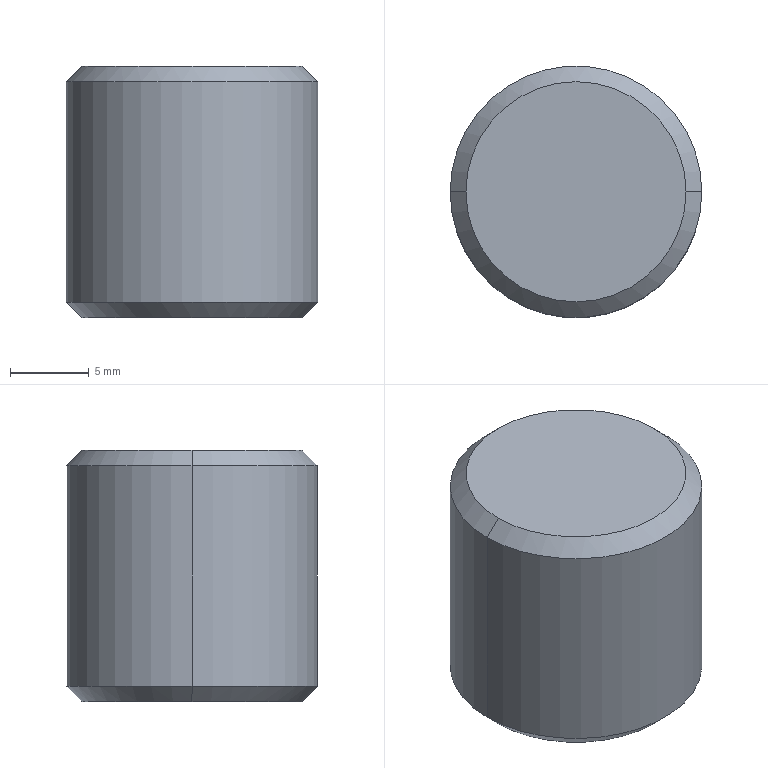Part | STEP file | SX-006-04 | 1 solid | 14 faces | box 16 x 16 x 16 mm | volume 2921 mm3 | cone 8 | cylinder 4 | plane 2 | commonest cylinder face diameters 5 x2 16 x2
STEP:
#1=CARTESIAN_POINT('',(0.,0.,0.));
#2=DIRECTION('',(0.,0.,1.));
#3=DIRECTION('',(1.,0.,0.));
#4=AXIS2_PLACEMENT_3D('',#1,#2,#3);
#5=CARTESIAN_POINT('',(-7.,0.,0.));
#6=VERTEX_POINT('',#5);
#7=CARTESIAN_POINT('',(7.,0.,0.));
#8=VERTEX_POINT('',#7);
#9=CARTESIAN_POINT('',(0.,0.,0.));
#10=DIRECTION('',(0.,0.,-1.));
#11=DIRECTION('',(1.,0.,0.));
#12=AXIS2_PLACEMENT_3D('',#9,#10,#11);
#13=CIRCLE('',#12,7.);
#14=CARTESIAN_POINT('',(0.,0.,1.));
#15=DIRECTION('',(0.,0.,1.));
#16=DIRECTION('',(1.,0.,0.));
#17=AXIS2_PLACEMENT_3D('',#14,#15,#16);
#18=CONICAL_SURFACE('',#17,8.,0.7854);
#19=CARTESIAN_POINT('',(6.283,-1.));
#20=DIRECTION('',(-1.,0.));
#21=VECTOR('',#20,1.);
#22=LINE('',#19,#21);
#23=(GEOMETRIC_REPRESENTATION_CONTEXT(2)PARAMETRIC_REPRESENTATION_CONTEXT()REPRESENTATION_CONTEXT('',''));
#24=DEFINITIONAL_REPRESENTATION('',(#22),#23);
#25=PCURVE('',#18,#24);
#26=CARTESIAN_POINT('',(0.,0.,0.));
#27=DIRECTION('',(0.,0.,1.));
#28=DIRECTION('',(1.,0.,0.));
#29=AXIS2_PLACEMENT_3D('',#26,#27,#28);
#30=PLANE('',#29);
#31=CARTESIAN_POINT('',(7.,0.));
#32=CARTESIAN_POINT('',(7.,-12.124));
#33=CARTESIAN_POINT('',(-3.5,-6.062));
#34=CARTESIAN_POINT('',(-14.,0.));
#35=CARTESIAN_POINT('',(-3.5,6.062));
#36=CARTESIAN_POINT('',(7.,12.124));
#37=CARTESIAN_POINT('',(7.,0.));
#38=(BOUNDED_CURVE()B_SPLINE_CURVE(2,(#31,#32,#33,#34,#35,#36,#37),.UNSPECIFIED.,.T.,.F.)B_SPLINE_CURVE_WITH_KNOTS((1,2,2,2,2,1),(-2.094,0.,2.094,4.189,6.283,8.378),.UNSPECIFIED.)CURVE()GEOMETRIC_REPRESENTATION_ITEM()RATIONAL_B_SPLINE_CURVE((1.,0.5,1.,0.5,1.,0.5,1.))REPRESENTATION_ITEM(''));
#39=(GEOMETRIC_REPRESENTATION_CONTEXT(2)PARAMETRIC_REPRESENTATION_CONTEXT()REPRESENTATION_CONTEXT('',''));
#40=DEFINITIONAL_REPRESENTATION('',(#38),#39);
#41=PCURVE('',#30,#40);
#42=SURFACE_CURVE('',#13,(#25,#41),.PCURVE_S1.);
#43=EDGE_CURVE('',#6,#8,#42,.T.);
#44=ORIENTED_EDGE('',*,*,#43,.F.);
#45=CARTESIAN_POINT('',(-8.,0.,1.));
#46=VERTEX_POINT('',#45);
#47=CARTESIAN_POINT('',(-8.,0.,1.));
#48=DIRECTION('',(-0.7071,0.,0.7071));
#49=VECTOR('',#48,1.);
#50=LINE('',#47,#49);
#51=CARTESIAN_POINT('',(3.142,0.));
#52=DIRECTION('',(0.,1.));
#53=VECTOR('',#52,1.);
#54=LINE('',#51,#53);
#55=(GEOMETRIC_REPRESENTATION_CONTEXT(2)PARAMETRIC_REPRESENTATION_CONTEXT()REPRESENTATION_CONTEXT('',''));
#56=DEFINITIONAL_REPRESENTATION('',(#54),#55);
#57=PCURVE('',#18,#56);
#58=CARTESIAN_POINT('',(0.,0.,1.));
#59=DIRECTION('',(0.,0.,1.));
#60=DIRECTION('',(1.,0.,0.));
#61=AXIS2_PLACEMENT_3D('',#58,#59,#60);
#62=CONICAL_SURFACE('',#61,8.,0.7854);
#63=CARTESIAN_POINT('',(3.142,0.));
#64=DIRECTION('',(0.,1.));
#65=VECTOR('',#64,1.);
#66=LINE('',#63,#65);
#67=(GEOMETRIC_REPRESENTATION_CONTEXT(2)PARAMETRIC_REPRESENTATION_CONTEXT()REPRESENTATION_CONTEXT('',''));
#68=DEFINITIONAL_REPRESENTATION('',(#66),#67);
#69=PCURVE('',#62,#68);
#70=SURFACE_CURVE('',#50,(#57,#69),.PCURVE_S1.);
#71=EDGE_CURVE('',#6,#46,#70,.T.);
#72=ORIENTED_EDGE('',*,*,#71,.T.);
#73=CARTESIAN_POINT('',(8.,0.,1.));
#74=VERTEX_POINT('',#73);
#75=CARTESIAN_POINT('',(0.,0.,1.));
#76=DIRECTION('',(0.,0.,1.));
#77=DIRECTION('',(1.,0.,0.));
#78=AXIS2_PLACEMENT_3D('',#75,#76,#77);
#79=CIRCLE('',#78,8.);
#80=CARTESIAN_POINT('',(0.,0.));
#81=DIRECTION('',(1.,0.));
#82=VECTOR('',#81,1.);
#83=LINE('',#80,#82);
#84=(GEOMETRIC_REPRESENTATION_CONTEXT(2)PARAMETRIC_REPRESENTATION_CONTEXT()REPRESENTATION_CONTEXT('',''));
#85=DEFINITIONAL_REPRESENTATION('',(#83),#84);
#86=PCURVE('',#18,#85);
#87=CARTESIAN_POINT('',(0.,0.,16.));
#88=DIRECTION('',(0.,0.,-1.));
#89=DIRECTION('',(-1.,0.,0.));
#90=AXIS2_PLACEMENT_3D('',#87,#88,#89);
#91=CYLINDRICAL_SURFACE('',#90,8.);
#92=CARTESIAN_POINT('',(3.142,15.));
#93=DIRECTION('',(-1.,0.));
#94=VECTOR('',#93,1.);
#95=LINE('',#92,#94);
#96=(GEOMETRIC_REPRESENTATION_CONTEXT(2)PARAMETRIC_REPRESENTATION_CONTEXT()REPRESENTATION_CONTEXT('',''));
#97=DEFINITIONAL_REPRESENTATION('',(#95),#96);
#98=PCURVE('',#91,#97);
#99=SURFACE_CURVE('',#79,(#86,#98),.PCURVE_S1.);
#100=EDGE_CURVE('',#74,#46,#99,.T.);
#101=ORIENTED_EDGE('',*,*,#100,.F.);
#102=CARTESIAN_POINT('',(8.,0.,1.));
#103=DIRECTION('',(0.7071,0.,0.7071));
#104=VECTOR('',#103,1.);
#105=LINE('',#102,#104);
#106=CARTESIAN_POINT('',(0.,0.));
#107=DIRECTION('',(0.,1.));
#108=VECTOR('',#107,1.);
#109=LINE('',#106,#108);
#110=(GEOMETRIC_REPRESENTATION_CONTEXT(2)PARAMETRIC_REPRESENTATION_CONTEXT()REPRESENTATION_CONTEXT('',''));
#111=DEFINITIONAL_REPRESENTATION('',(#109),#110);
#112=PCURVE('',#18,#111);
#113=CARTESIAN_POINT('',(6.283,0.));
#114=DIRECTION('',(0.,1.));
#115=VECTOR('',#114,1.);
#116=LINE('',#113,#115);
#117=(GEOMETRIC_REPRESENTATION_CONTEXT(2)PARAMETRIC_REPRESENTATION_CONTEXT()REPRESENTATION_CONTEXT('',''));
#118=DEFINITIONAL_REPRESENTATION('',(#116),#117);
#119=PCURVE('',#62,#118);
#120=SURFACE_CURVE('',#105,(#112,#119),.PCURVE_S1.);
#121=EDGE_CURVE('',#8,#74,#120,.T.);
#122=ORIENTED_EDGE('',*,*,#121,.F.);
#123=EDGE_LOOP('',(#44,#72,#101,#122));
#124=FACE_BOUND('',#123,.T.);
#125=ADVANCED_FACE('',(#124),#18,.T.);
#126=CARTESIAN_POINT('',(7.,0.,16.));
#127=VERTEX_POINT('',#126);
#128=CARTESIAN_POINT('',(-7.,0.,16.));
#129=VERTEX_POINT('',#128);
#130=CARTESIAN_POINT('',(0.,0.,16.));
#131=DIRECTION('',(0.,0.,1.));
#132=DIRECTION('',(1.,0.,0.));
#133=AXIS2_PLACEMENT_3D('',#130,#131,#132);
#134=CIRCLE('',#133,7.);
#135=CARTESIAN_POINT('',(0.,0.,16.));
#136=DIRECTION('',(0.,0.,-1.));
#137=DIRECTION('',(-1.,0.,0.));
#138=AXIS2_PLACEMENT_3D('',#135,#136,#137);
#139=CONICAL_SURFACE('',#138,7.,0.7854);
#140=CARTESIAN_POINT('',(3.142,0.));
#141=DIRECTION('',(-1.,0.));
#142=VECTOR('',#141,1.);
#143=LINE('',#140,#142);
#144=(GEOMETRIC_REPRESENTATION_CONTEXT(2)PARAMETRIC_REPRESENTATION_CONTEXT()REPRESENTATION_CONTEXT('',''));
#145=DEFINITIONAL_REPRESENTATION('',(#143),#144);
#146=PCURVE('',#139,#145);
#147=CARTESIAN_POINT('',(0.,0.,16.));
#148=DIRECTION('',(0.,0.,1.));
#149=DIRECTION('',(1.,0.,0.));
#150=AXIS2_PLACEMENT_3D('',#147,#148,#149);
#151=PLANE('',#150);
#152=CARTESIAN_POINT('',(0.,0.));
#153=DIRECTION('',(1.,0.));
#154=AXIS2_PLACEMENT_2D('',#152,#153);
#155=CIRCLE('',#154,7.);
#156=(GEOMETRIC_REPRESENTATION_CONTEXT(2)PARAMETRIC_REPRESENTATION_CONTEXT()REPRESENTATION_CONTEXT('',''));
#157=DEFINITIONAL_REPRESENTATION('',(#155),#156);
#158=PCURVE('',#151,#157);
#159=SURFACE_CURVE('',#134,(#146,#158),.PCURVE_S1.);
#160=EDGE_CURVE('',#127,#129,#159,.T.);
#161=ORIENTED_EDGE('',*,*,#160,.F.);
#162=CARTESIAN_POINT('',(8.,0.,15.));
#163=VERTEX_POINT('',#162);
#164=CARTESIAN_POINT('',(7.,0.,16.));
#165=DIRECTION('',(0.7071,0.,-0.7071));
#166=VECTOR('',#165,1.);
#167=LINE('',#164,#166);
#168=CARTESIAN_POINT('',(3.142,0.));
#169=DIRECTION('',(0.,1.));
#170=VECTOR('',#169,1.);
#171=LINE('',#168,#170);
#172=(GEOMETRIC_REPRESENTATION_CONTEXT(2)PARAMETRIC_REPRESENTATION_CONTEXT()REPRESENTATION_CONTEXT('',''));
#173=DEFINITIONAL_REPRESENTATION('',(#171),#172);
#174=PCURVE('',#139,#173);
#175=CARTESIAN_POINT('',(0.,0.,16.));
#176=DIRECTION('',(0.,0.,-1.));
#177=DIRECTION('',(-1.,0.,0.));
#178=AXIS2_PLACEMENT_3D('',#175,#176,#177);
#179=CONICAL_SURFACE('',#178,7.,0.7854);
#180=CARTESIAN_POINT('',(3.142,0.));
#181=DIRECTION('',(0.,1.));
#182=VECTOR('',#181,1.);
#183=LINE('',#180,#182);
#184=(GEOMETRIC_REPRESENTATION_CONTEXT(2)PARAMETRIC_REPRESENTATION_CONTEXT()REPRESENTATION_CONTEXT('',''));
#185=DEFINITIONAL_REPRESENTATION('',(#183),#184);
#186=PCURVE('',#179,#185);
#187=SURFACE_CURVE('',#167,(#174,#186),.PCURVE_S1.);
#188=EDGE_CURVE('',#127,#163,#187,.T.);
#189=ORIENTED_EDGE('',*,*,#188,.T.);
#190=CARTESIAN_POINT('',(-8.,0.,15.));
#191=VERTEX_POINT('',#190);
#192=CARTESIAN_POINT('',(0.,0.,15.));
#193=DIRECTION('',(0.,0.,-1.));
#194=DIRECTION('',(1.,0.,0.));
#195=AXIS2_PLACEMENT_3D('',#192,#193,#194);
#196=CIRCLE('',#195,8.);
#197=CARTESIAN_POINT('',(-3.142,1.));
#198=DIRECTION('',(1.,0.));
#199=VECTOR('',#198,1.);
#200=LINE('',#197,#199);
#201=(GEOMETRIC_REPRESENTATION_CONTEXT(2)PARAMETRIC_REPRESENTATION_CONTEXT()REPRESENTATION_CONTEXT('',''));
#202=DEFINITIONAL_REPRESENTATION('',(#200),#201);
#203=PCURVE('',#139,#202);
#204=CARTESIAN_POINT('',(-3.142,1.));
#205=DIRECTION('',(1.,0.));
#206=VECTOR('',#205,1.);
#207=LINE('',#204,#206);
#208=(GEOMETRIC_REPRESENTATION_CONTEXT(2)PARAMETRIC_REPRESENTATION_CONTEXT()REPRESENTATION_CONTEXT('',''));
#209=DEFINITIONAL_REPRESENTATION('',(#207),#208);
#210=PCURVE('',#91,#209);
#211=SURFACE_CURVE('',#196,(#203,#210),.PCURVE_S1.);
#212=EDGE_CURVE('',#191,#163,#211,.T.);
#213=ORIENTED_EDGE('',*,*,#212,.F.);
#214=CARTESIAN_POINT('',(-7.,0.,16.));
#215=DIRECTION('',(-0.7071,0.,-0.7071));
#216=VECTOR('',#215,1.);
#217=LINE('',#214,#216);
#218=CARTESIAN_POINT('',(0.,0.));
#219=DIRECTION('',(0.,1.));
#220=VECTOR('',#219,1.);
#221=LINE('',#218,#220);
#222=(GEOMETRIC_REPRESENTATION_CONTEXT(2)PARAMETRIC_REPRESENTATION_CONTEXT()REPRESENTATION_CONTEXT('',''));
#223=DEFINITIONAL_REPRESENTATION('',(#221),#222);
#224=PCURVE('',#139,#223);
#225=CARTESIAN_POINT('',(6.283,0.));
#226=DIRECTION('',(0.,1.));
#227=VECTOR('',#226,1.);
#228=LINE('',#225,#227);
#229=(GEOMETRIC_REPRESENTATION_CONTEXT(2)PARAMETRIC_REPRESENTATION_CONTEXT()REPRESENTATION_CONTEXT('',''));
#230=DEFINITIONAL_REPRESENTATION('',(#228),#229);
#231=PCURVE('',#179,#230);
#232=SURFACE_CURVE('',#217,(#224,#231),.PCURVE_S1.);
#233=EDGE_CURVE('',#129,#191,#232,.T.);
#234=ORIENTED_EDGE('',*,*,#233,.F.);
#235=EDGE_LOOP('',(#161,#189,#213,#234));
#236=FACE_BOUND('',#235,.T.);
#237=ADVANCED_FACE('',(#236),#139,.T.);
#238=CARTESIAN_POINT('',(-2.5,0.,0.525));
#239=VERTEX_POINT('',#238);
#240=CARTESIAN_POINT('',(-3.025,0.,0.));
#241=VERTEX_POINT('',#240);
#242=CARTESIAN_POINT('',(-3.025,0.,0.));
#243=DIRECTION('',(-0.7071,0.,-0.7071));
#244=VECTOR('',#243,1.);
#245=LINE('',#242,#244);
#246=CARTESIAN_POINT('',(0.,0.,0.));
#247=DIRECTION('',(0.,0.,-1.));
#248=DIRECTION('',(-1.,0.,0.));
#249=AXIS2_PLACEMENT_3D('',#246,#247,#248);
#250=CONICAL_SURFACE('',#249,3.025,0.7854);
#251=CARTESIAN_POINT('',(6.283,0.));
#252=DIRECTION('',(0.,1.));
#253=VECTOR('',#252,1.);
#254=LINE('',#251,#253);
#255=(GEOMETRIC_REPRESENTATION_CONTEXT(2)PARAMETRIC_REPRESENTATION_CONTEXT()REPRESENTATION_CONTEXT('',''));
#256=DEFINITIONAL_REPRESENTATION('',(#254),#255);
#257=PCURVE('',#250,#256);
#258=CARTESIAN_POINT('',(0.,0.,0.));
#259=DIRECTION('',(0.,0.,-1.));
#260=DIRECTION('',(-1.,0.,0.));
#261=AXIS2_PLACEMENT_3D('',#258,#259,#260);
#262=CONICAL_SURFACE('',#261,3.025,0.7854);
#263=CARTESIAN_POINT('',(0.,0.));
#264=DIRECTION('',(0.,1.));
#265=VECTOR('',#264,1.);
#266=LINE('',#263,#265);
#267=(GEOMETRIC_REPRESENTATION_CONTEXT(2)PARAMETRIC_REPRESENTATION_CONTEXT()REPRESENTATION_CONTEXT('',''));
#268=DEFINITIONAL_REPRESENTATION('',(#266),#267);
#269=PCURVE('',#262,#268);
#270=SURFACE_CURVE('',#245,(#257,#269),.PCURVE_S1.);
#271=EDGE_CURVE('',#239,#241,#270,.T.);
#272=ORIENTED_EDGE('',*,*,#271,.T.);
#273=CARTESIAN_POINT('',(3.025,0.,0.));
#274=VERTEX_POINT('',#273);
#275=CARTESIAN_POINT('',(0.,0.,0.));
#276=DIRECTION('',(0.,0.,-1.));
#277=DIRECTION('',(-1.,0.,0.));
#278=AXIS2_PLACEMENT_3D('',#275,#276,#277);
#279=CIRCLE('',#278,3.025);
#280=CARTESIAN_POINT('',(0.,0.));
#281=DIRECTION('',(1.,0.));
#282=VECTOR('',#281,1.);
#283=LINE('',#280,#282);
#284=(GEOMETRIC_REPRESENTATION_CONTEXT(2)PARAMETRIC_REPRESENTATION_CONTEXT()REPRESENTATION_CONTEXT('',''));
#285=DEFINITIONAL_REPRESENTATION('',(#283),#284);
#286=PCURVE('',#250,#285);
#287=CARTESIAN_POINT('',(-3.025,0.));
#288=CARTESIAN_POINT('',(-3.025,5.239));
#289=CARTESIAN_POINT('',(1.512,2.62));
#290=CARTESIAN_POINT('',(6.05,0.));
#291=CARTESIAN_POINT('',(1.512,-2.62));
#292=CARTESIAN_POINT('',(-3.025,-5.239));
#293=CARTESIAN_POINT('',(-3.025,0.));
#294=(BOUNDED_CURVE()B_SPLINE_CURVE(2,(#287,#288,#289,#290,#291,#292,#293),.UNSPECIFIED.,.T.,.F.)B_SPLINE_CURVE_WITH_KNOTS((1,2,2,2,2,1),(-2.094,0.,2.094,4.189,6.283,8.378),.UNSPECIFIED.)CURVE()GEOMETRIC_REPRESENTATION_ITEM()RATIONAL_B_SPLINE_CURVE((1.,0.5,1.,0.5,1.,0.5,1.))REPRESENTATION_ITEM(''));
#295=(GEOMETRIC_REPRESENTATION_CONTEXT(2)PARAMETRIC_REPRESENTATION_CONTEXT()REPRESENTATION_CONTEXT('',''));
#296=DEFINITIONAL_REPRESENTATION('',(#294),#295);
#297=PCURVE('',#30,#296);
#298=SURFACE_CURVE('',#279,(#286,#297),.PCURVE_S1.);
#299=EDGE_CURVE('',#274,#241,#298,.T.);
#300=ORIENTED_EDGE('',*,*,#299,.F.);
#301=CARTESIAN_POINT('',(2.5,0.,0.525));
#302=VERTEX_POINT('',#301);
#303=CARTESIAN_POINT('',(3.025,0.,0.));
#304=DIRECTION('',(0.7071,0.,-0.7071));
#305=VECTOR('',#304,1.);
#306=LINE('',#303,#305);
#307=CARTESIAN_POINT('',(3.142,0.));
#308=DIRECTION('',(0.,1.));
#309=VECTOR('',#308,1.);
#310=LINE('',#307,#309);
#311=(GEOMETRIC_REPRESENTATION_CONTEXT(2)PARAMETRIC_REPRESENTATION_CONTEXT()REPRESENTATION_CONTEXT('',''));
#312=DEFINITIONAL_REPRESENTATION('',(#310),#311);
#313=PCURVE('',#250,#312);
#314=CARTESIAN_POINT('',(3.142,0.));
#315=DIRECTION('',(0.,1.));
#316=VECTOR('',#315,1.);
#317=LINE('',#314,#316);
#318=(GEOMETRIC_REPRESENTATION_CONTEXT(2)PARAMETRIC_REPRESENTATION_CONTEXT()REPRESENTATION_CONTEXT('',''));
#319=DEFINITIONAL_REPRESENTATION('',(#317),#318);
#320=PCURVE('',#262,#319);
#321=SURFACE_CURVE('',#306,(#313,#320),.PCURVE_S1.);
#322=EDGE_CURVE('',#302,#274,#321,.T.);
#323=ORIENTED_EDGE('',*,*,#322,.F.);
#324=CARTESIAN_POINT('',(0.,0.,0.525));
#325=DIRECTION('',(0.,0.,-1.));
#326=DIRECTION('',(-1.,0.,0.));
#327=AXIS2_PLACEMENT_3D('',#324,#325,#326);
#328=CIRCLE('',#327,2.5);
#329=CARTESIAN_POINT('',(0.,-0.525));
#330=DIRECTION('',(1.,0.));
#331=VECTOR('',#330,1.);
#332=LINE('',#329,#331);
#333=(GEOMETRIC_REPRESENTATION_CONTEXT(2)PARAMETRIC_REPRESENTATION_CONTEXT()REPRESENTATION_CONTEXT('',''));
#334=DEFINITIONAL_REPRESENTATION('',(#332),#333);
#335=PCURVE('',#250,#334);
#336=CARTESIAN_POINT('',(0.,0.,0.));
#337=DIRECTION('',(0.,0.,-1.));
#338=DIRECTION('',(-1.,0.,0.));
#339=AXIS2_PLACEMENT_3D('',#336,#337,#338);
#340=CYLINDRICAL_SURFACE('',#339,2.5);
#341=CARTESIAN_POINT('',(0.,-0.525));
#342=DIRECTION('',(1.,0.));
#343=VECTOR('',#342,1.);
#344=LINE('',#341,#343);
#345=(GEOMETRIC_REPRESENTATION_CONTEXT(2)PARAMETRIC_REPRESENTATION_CONTEXT()REPRESENTATION_CONTEXT('',''));
#346=DEFINITIONAL_REPRESENTATION('',(#344),#345);
#347=PCURVE('',#340,#346);
#348=SURFACE_CURVE('',#328,(#335,#347),.PCURVE_S1.);
#349=EDGE_CURVE('',#302,#239,#348,.T.);
#350=ORIENTED_EDGE('',*,*,#349,.T.);
#351=EDGE_LOOP('',(#272,#300,#323,#350));
#352=FACE_BOUND('',#351,.F.);
#353=ADVANCED_FACE('',(#352),#250,.F.);
#354=CARTESIAN_POINT('',(-2.5,0.,12.));
#355=VERTEX_POINT('',#354);
#356=CARTESIAN_POINT('',(-2.5,0.,0.));
#357=DIRECTION('',(0.,0.,-1.));
#358=VECTOR('',#357,1.);
#359=LINE('',#356,#358);
#360=CARTESIAN_POINT('',(6.283,0.));
#361=DIRECTION('',(0.,1.));
#362=VECTOR('',#361,1.);
#363=LINE('',#360,#362);
#364=(GEOMETRIC_REPRESENTATION_CONTEXT(2)PARAMETRIC_REPRESENTATION_CONTEXT()REPRESENTATION_CONTEXT('',''));
#365=DEFINITIONAL_REPRESENTATION('',(#363),#364);
#366=PCURVE('',#340,#365);
#367=CARTESIAN_POINT('',(0.,0.,0.));
#368=DIRECTION('',(0.,0.,-1.));
#369=DIRECTION('',(-1.,0.,0.));
#370=AXIS2_PLACEMENT_3D('',#367,#368,#369);
#371=CYLINDRICAL_SURFACE('',#370,2.5);
#372=CARTESIAN_POINT('',(0.,0.));
#373=DIRECTION('',(0.,1.));
#374=VECTOR('',#373,1.);
#375=LINE('',#372,#374);
#376=(GEOMETRIC_REPRESENTATION_CONTEXT(2)PARAMETRIC_REPRESENTATION_CONTEXT()REPRESENTATION_CONTEXT('',''));
#377=DEFINITIONAL_REPRESENTATION('',(#375),#376);
#378=PCURVE('',#371,#377);
#379=SURFACE_CURVE('',#359,(#366,#378),.PCURVE_S1.);
#380=EDGE_CURVE('',#355,#239,#379,.T.);
#381=ORIENTED_EDGE('',*,*,#380,.T.);
#382=ORIENTED_EDGE('',*,*,#349,.F.);
#383=CARTESIAN_POINT('',(2.5,0.,12.));
#384=VERTEX_POINT('',#383);
#385=CARTESIAN_POINT('',(2.5,0.,0.));
#386=DIRECTION('',(0.,0.,-1.));
#387=VECTOR('',#386,1.);
#388=LINE('',#385,#387);
#389=CARTESIAN_POINT('',(3.142,0.));
#390=DIRECTION('',(0.,1.));
#391=VECTOR('',#390,1.);
#392=LINE('',#389,#391);
#393=(GEOMETRIC_REPRESENTATION_CONTEXT(2)PARAMETRIC_REPRESENTATION_CONTEXT()REPRESENTATION_CONTEXT('',''));
#394=DEFINITIONAL_REPRESENTATION('',(#392),#393);
#395=PCURVE('',#340,#394);
#396=CARTESIAN_POINT('',(3.142,0.));
#397=DIRECTION('',(0.,1.));
#398=VECTOR('',#397,1.);
#399=LINE('',#396,#398);
#400=(GEOMETRIC_REPRESENTATION_CONTEXT(2)PARAMETRIC_REPRESENTATION_CONTEXT()REPRESENTATION_CONTEXT('',''));
#401=DEFINITIONAL_REPRESENTATION('',(#399),#400);
#402=PCURVE('',#371,#401);
#403=SURFACE_CURVE('',#388,(#395,#402),.PCURVE_S1.);
#404=EDGE_CURVE('',#384,#302,#403,.T.);
#405=ORIENTED_EDGE('',*,*,#404,.F.);
#406=CARTESIAN_POINT('',(0.,0.,12.));
#407=DIRECTION('',(0.,0.,-1.));
#408=DIRECTION('',(-1.,0.,0.));
#409=AXIS2_PLACEMENT_3D('',#406,#407,#408);
#410=CIRCLE('',#409,2.5);
#411=CARTESIAN_POINT('',(0.,-12.));
#412=DIRECTION('',(1.,0.));
#413=VECTOR('',#412,1.);
#414=LINE('',#411,#413);
#415=(GEOMETRIC_REPRESENTATION_CONTEXT(2)PARAMETRIC_REPRESENTATION_CONTEXT()REPRESENTATION_CONTEXT('',''));
#416=DEFINITIONAL_REPRESENTATION('',(#414),#415);
#417=PCURVE('',#340,#416);
#418=CARTESIAN_POINT('',(0.,0.,12.));
#419=DIRECTION('',(0.,0.,-1.));
#420=DIRECTION('',(-1.,0.,0.));
#421=AXIS2_PLACEMENT_3D('',#418,#419,#420);
#422=CONICAL_SURFACE('',#421,2.5,1.03);
#423=CARTESIAN_POINT('',(0.,0.));
#424=DIRECTION('',(1.,0.));
#425=VECTOR('',#424,1.);
#426=LINE('',#423,#425);
#427=(GEOMETRIC_REPRESENTATION_CONTEXT(2)PARAMETRIC_REPRESENTATION_CONTEXT()REPRESENTATION_CONTEXT('',''));
#428=DEFINITIONAL_REPRESENTATION('',(#426),#427);
#429=PCURVE('',#422,#428);
#430=SURFACE_CURVE('',#410,(#417,#429),.PCURVE_S1.);
#431=EDGE_CURVE('',#384,#355,#430,.T.);
#432=ORIENTED_EDGE('',*,*,#431,.T.);
#433=EDGE_LOOP('',(#381,#382,#405,#432));
#434=FACE_BOUND('',#433,.F.);
#435=ADVANCED_FACE('',(#434),#340,.F.);
#436=ORIENTED_EDGE('',*,*,#431,.F.);
#437=CARTESIAN_POINT('',(0.,0.,13.502));
#438=VERTEX_POINT('',#437);
#439=CARTESIAN_POINT('',(2.5,0.,12.));
#440=DIRECTION('',(0.8572,0.,-0.515));
#441=VECTOR('',#440,1.);
#442=LINE('',#439,#441);
#443=CARTESIAN_POINT('',(3.142,0.));
#444=DIRECTION('',(0.,1.));
#445=VECTOR('',#444,1.);
#446=LINE('',#443,#445);
#447=(GEOMETRIC_REPRESENTATION_CONTEXT(2)PARAMETRIC_REPRESENTATION_CONTEXT()REPRESENTATION_CONTEXT('',''));
#448=DEFINITIONAL_REPRESENTATION('',(#446),#447);
#449=PCURVE('',#422,#448);
#450=CARTESIAN_POINT('',(0.,0.,12.));
#451=DIRECTION('',(0.,0.,-1.));
#452=DIRECTION('',(-1.,0.,0.));
#453=AXIS2_PLACEMENT_3D('',#450,#451,#452);
#454=CONICAL_SURFACE('',#453,2.5,1.03);
#455=CARTESIAN_POINT('',(3.142,0.));
#456=DIRECTION('',(0.,1.));
#457=VECTOR('',#456,1.);
#458=LINE('',#455,#457);
#459=(GEOMETRIC_REPRESENTATION_CONTEXT(2)PARAMETRIC_REPRESENTATION_CONTEXT()REPRESENTATION_CONTEXT('',''));
#460=DEFINITIONAL_REPRESENTATION('',(#458),#459);
#461=PCURVE('',#454,#460);
#462=SURFACE_CURVE('',#442,(#449,#461),.PCURVE_S1.);
#463=EDGE_CURVE('',#438,#384,#462,.T.);
#464=ORIENTED_EDGE('',*,*,#463,.F.);
#465=CARTESIAN_POINT('',(-2.5,0.,12.));
#466=DIRECTION('',(-0.8572,0.,-0.515));
#467=VECTOR('',#466,1.);
#468=LINE('',#465,#467);
#469=CARTESIAN_POINT('',(6.283,0.));
#470=DIRECTION('',(0.,1.));
#471=VECTOR('',#470,1.);
#472=LINE('',#469,#471);
#473=(GEOMETRIC_REPRESENTATION_CONTEXT(2)PARAMETRIC_REPRESENTATION_CONTEXT()REPRESENTATION_CONTEXT('',''));
#474=DEFINITIONAL_REPRESENTATION('',(#472),#473);
#475=PCURVE('',#422,#474);
#476=CARTESIAN_POINT('',(0.,0.));
#477=DIRECTION('',(0.,1.));
#478=VECTOR('',#477,1.);
#479=LINE('',#476,#478);
#480=(GEOMETRIC_REPRESENTATION_CONTEXT(2)PARAMETRIC_REPRESENTATION_CONTEXT()REPRESENTATION_CONTEXT('',''));
#481=DEFINITIONAL_REPRESENTATION('',(#479),#480);
#482=PCURVE('',#454,#481);
#483=SURFACE_CURVE('',#468,(#475,#482),.PCURVE_S1.);
#484=EDGE_CURVE('',#438,#355,#483,.T.);
#485=ORIENTED_EDGE('',*,*,#484,.T.);
#486=EDGE_LOOP('',(#436,#464,#485));
#487=FACE_BOUND('',#486,.F.);
#488=ADVANCED_FACE('',(#487),#422,.F.);
#489=ORIENTED_EDGE('',*,*,#212,.T.);
#490=CARTESIAN_POINT('',(8.,0.,16.));
#491=DIRECTION('',(0.,0.,-1.));
#492=VECTOR('',#491,1.);
#493=LINE('',#490,#492);
#494=CARTESIAN_POINT('',(3.142,0.));
#495=DIRECTION('',(0.,1.));
#496=VECTOR('',#495,1.);
#497=LINE('',#494,#496);
#498=(GEOMETRIC_REPRESENTATION_CONTEXT(2)PARAMETRIC_REPRESENTATION_CONTEXT()REPRESENTATION_CONTEXT('',''));
#499=DEFINITIONAL_REPRESENTATION('',(#497),#498);
#500=PCURVE('',#91,#499);
#501=CARTESIAN_POINT('',(0.,0.,16.));
#502=DIRECTION('',(0.,0.,-1.));
#503=DIRECTION('',(-1.,0.,0.));
#504=AXIS2_PLACEMENT_3D('',#501,#502,#503);
#505=CYLINDRICAL_SURFACE('',#504,8.);
#506=CARTESIAN_POINT('',(3.142,0.));
#507=DIRECTION('',(0.,1.));
#508=VECTOR('',#507,1.);
#509=LINE('',#506,#508);
#510=(GEOMETRIC_REPRESENTATION_CONTEXT(2)PARAMETRIC_REPRESENTATION_CONTEXT()REPRESENTATION_CONTEXT('',''));
#511=DEFINITIONAL_REPRESENTATION('',(#509),#510);
#512=PCURVE('',#505,#511);
#513=SURFACE_CURVE('',#493,(#500,#512),.PCURVE_S1.);
#514=EDGE_CURVE('',#163,#74,#513,.T.);
#515=ORIENTED_EDGE('',*,*,#514,.T.);
#516=ORIENTED_EDGE('',*,*,#100,.T.);
#517=CARTESIAN_POINT('',(-8.,0.,16.));
#518=DIRECTION('',(0.,0.,-1.));
#519=VECTOR('',#518,1.);
#520=LINE('',#517,#519);
#521=CARTESIAN_POINT('',(0.,0.));
#522=DIRECTION('',(0.,1.));
#523=VECTOR('',#522,1.);
#524=LINE('',#521,#523);
#525=(GEOMETRIC_REPRESENTATION_CONTEXT(2)PARAMETRIC_REPRESENTATION_CONTEXT()REPRESENTATION_CONTEXT('',''));
#526=DEFINITIONAL_REPRESENTATION('',(#524),#525);
#527=PCURVE('',#91,#526);
#528=CARTESIAN_POINT('',(6.283,0.));
#529=DIRECTION('',(0.,1.));
#530=VECTOR('',#529,1.);
#531=LINE('',#528,#530);
#532=(GEOMETRIC_REPRESENTATION_CONTEXT(2)PARAMETRIC_REPRESENTATION_CONTEXT()REPRESENTATION_CONTEXT('',''));
#533=DEFINITIONAL_REPRESENTATION('',(#531),#532);
#534=PCURVE('',#505,#533);
#535=SURFACE_CURVE('',#520,(#527,#534),.PCURVE_S1.);
#536=EDGE_CURVE('',#191,#46,#535,.T.);
#537=ORIENTED_EDGE('',*,*,#536,.F.);
#538=EDGE_LOOP('',(#489,#515,#516,#537));
#539=FACE_BOUND('',#538,.T.);
#540=ADVANCED_FACE('',(#539),#91,.T.);
#541=ORIENTED_EDGE('',*,*,#514,.F.);
#542=CARTESIAN_POINT('',(0.,0.,15.));
#543=DIRECTION('',(0.,0.,-1.));
#544=DIRECTION('',(1.,0.,0.));
#545=AXIS2_PLACEMENT_3D('',#542,#543,#544);
#546=CIRCLE('',#545,8.);
#547=CARTESIAN_POINT('',(3.142,1.));
#548=DIRECTION('',(1.,0.));
#549=VECTOR('',#548,1.);
#550=LINE('',#547,#549);
#551=(GEOMETRIC_REPRESENTATION_CONTEXT(2)PARAMETRIC_REPRESENTATION_CONTEXT()REPRESENTATION_CONTEXT('',''));
#552=DEFINITIONAL_REPRESENTATION('',(#550),#551);
#553=PCURVE('',#505,#552);
#554=CARTESIAN_POINT('',(3.142,1.));
#555=DIRECTION('',(1.,0.));
#556=VECTOR('',#555,1.);
#557=LINE('',#554,#556);
#558=(GEOMETRIC_REPRESENTATION_CONTEXT(2)PARAMETRIC_REPRESENTATION_CONTEXT()REPRESENTATION_CONTEXT('',''));
#559=DEFINITIONAL_REPRESENTATION('',(#557),#558);
#560=PCURVE('',#179,#559);
#561=SURFACE_CURVE('',#546,(#553,#560),.PCURVE_S1.);
#562=EDGE_CURVE('',#163,#191,#561,.T.);
#563=ORIENTED_EDGE('',*,*,#562,.T.);
#564=ORIENTED_EDGE('',*,*,#536,.T.);
#565=CARTESIAN_POINT('',(0.,0.,1.));
#566=DIRECTION('',(0.,0.,1.));
#567=DIRECTION('',(1.,0.,0.));
#568=AXIS2_PLACEMENT_3D('',#565,#566,#567);
#569=CIRCLE('',#568,8.);
#570=CARTESIAN_POINT('',(9.425,15.));
#571=DIRECTION('',(-1.,0.));
#572=VECTOR('',#571,1.);
#573=LINE('',#570,#572);
#574=(GEOMETRIC_REPRESENTATION_CONTEXT(2)PARAMETRIC_REPRESENTATION_CONTEXT()REPRESENTATION_CONTEXT('',''));
#575=DEFINITIONAL_REPRESENTATION('',(#573),#574);
#576=PCURVE('',#505,#575);
#577=CARTESIAN_POINT('',(0.,0.));
#578=DIRECTION('',(1.,0.));
#579=VECTOR('',#578,1.);
#580=LINE('',#577,#579);
#581=(GEOMETRIC_REPRESENTATION_CONTEXT(2)PARAMETRIC_REPRESENTATION_CONTEXT()REPRESENTATION_CONTEXT('',''));
#582=DEFINITIONAL_REPRESENTATION('',(#580),#581);
#583=PCURVE('',#62,#582);
#584=SURFACE_CURVE('',#569,(#576,#583),.PCURVE_S1.);
#585=EDGE_CURVE('',#46,#74,#584,.T.);
#586=ORIENTED_EDGE('',*,*,#585,.T.);
#587=EDGE_LOOP('',(#541,#563,#564,#586));
#588=FACE_BOUND('',#587,.T.);
#589=ADVANCED_FACE('',(#588),#505,.T.);
#590=CARTESIAN_POINT('',(0.,0.,16.));
#591=DIRECTION('',(0.,0.,1.));
#592=DIRECTION('',(1.,0.,0.));
#593=AXIS2_PLACEMENT_3D('',#590,#591,#592);
#594=CIRCLE('',#593,7.);
#595=CARTESIAN_POINT('',(0.,0.));
#596=DIRECTION('',(1.,0.));
#597=AXIS2_PLACEMENT_2D('',#595,#596);
#598=CIRCLE('',#597,7.);
#599=(GEOMETRIC_REPRESENTATION_CONTEXT(2)PARAMETRIC_REPRESENTATION_CONTEXT()REPRESENTATION_CONTEXT('',''));
#600=DEFINITIONAL_REPRESENTATION('',(#598),#599);
#601=PCURVE('',#151,#600);
#602=CARTESIAN_POINT('',(9.425,0.));
#603=DIRECTION('',(-1.,0.));
#604=VECTOR('',#603,1.);
#605=LINE('',#602,#604);
#606=(GEOMETRIC_REPRESENTATION_CONTEXT(2)PARAMETRIC_REPRESENTATION_CONTEXT()REPRESENTATION_CONTEXT('',''));
#607=DEFINITIONAL_REPRESENTATION('',(#605),#606);
#608=PCURVE('',#179,#607);
#609=SURFACE_CURVE('',#594,(#601,#608),.PCURVE_S1.);
#610=EDGE_CURVE('',#129,#127,#609,.T.);
#611=ORIENTED_EDGE('',*,*,#610,.T.);
#612=ORIENTED_EDGE('',*,*,#160,.T.);
#613=EDGE_LOOP('',(#611,#612));
#614=FACE_BOUND('',#613,.T.);
#615=ADVANCED_FACE('',(#614),#151,.T.);
#616=CARTESIAN_POINT('',(0.,0.,0.));
#617=DIRECTION('',(0.,0.,-1.));
#618=DIRECTION('',(1.,0.,0.));
#619=AXIS2_PLACEMENT_3D('',#616,#617,#618);
#620=CIRCLE('',#619,7.);
#621=CARTESIAN_POINT('',(7.,0.));
#622=CARTESIAN_POINT('',(7.,-12.124));
#623=CARTESIAN_POINT('',(-3.5,-6.062));
#624=CARTESIAN_POINT('',(-14.,0.));
#625=CARTESIAN_POINT('',(-3.5,6.062));
#626=CARTESIAN_POINT('',(7.,12.124));
#627=CARTESIAN_POINT('',(7.,0.));
#628=(BOUNDED_CURVE()B_SPLINE_CURVE(2,(#621,#622,#623,#624,#625,#626,#627),.UNSPECIFIED.,.T.,.F.)B_SPLINE_CURVE_WITH_KNOTS((1,2,2,2,2,1),(-2.094,0.,2.094,4.189,6.283,8.378),.UNSPECIFIED.)CURVE()GEOMETRIC_REPRESENTATION_ITEM()RATIONAL_B_SPLINE_CURVE((1.,0.5,1.,0.5,1.,0.5,1.))REPRESENTATION_ITEM(''));
#629=(GEOMETRIC_REPRESENTATION_CONTEXT(2)PARAMETRIC_REPRESENTATION_CONTEXT()REPRESENTATION_CONTEXT('',''));
#630=DEFINITIONAL_REPRESENTATION('',(#628),#629);
#631=PCURVE('',#30,#630);
#632=CARTESIAN_POINT('',(6.283,-1.));
#633=DIRECTION('',(-1.,0.));
#634=VECTOR('',#633,1.);
#635=LINE('',#632,#634);
#636=(GEOMETRIC_REPRESENTATION_CONTEXT(2)PARAMETRIC_REPRESENTATION_CONTEXT()REPRESENTATION_CONTEXT('',''));
#637=DEFINITIONAL_REPRESENTATION('',(#635),#636);
#638=PCURVE('',#62,#637);
#639=SURFACE_CURVE('',#620,(#631,#638),.PCURVE_S1.);
#640=EDGE_CURVE('',#8,#6,#639,.T.);
#641=ORIENTED_EDGE('',*,*,#640,.T.);
#642=ORIENTED_EDGE('',*,*,#43,.T.);
#643=EDGE_LOOP('',(#641,#642));
#644=FACE_BOUND('',#643,.T.);
#645=CARTESIAN_POINT('',(0.,0.,0.));
#646=DIRECTION('',(0.,0.,-1.));
#647=DIRECTION('',(-1.,0.,0.));
#648=AXIS2_PLACEMENT_3D('',#645,#646,#647);
#649=CIRCLE('',#648,3.025);
#650=CARTESIAN_POINT('',(-3.025,0.));
#651=CARTESIAN_POINT('',(-3.025,5.239));
#652=CARTESIAN_POINT('',(1.512,2.62));
#653=CARTESIAN_POINT('',(6.05,0.));
#654=CARTESIAN_POINT('',(1.512,-2.62));
#655=CARTESIAN_POINT('',(-3.025,-5.239));
#656=CARTESIAN_POINT('',(-3.025,0.));
#657=(BOUNDED_CURVE()B_SPLINE_CURVE(2,(#650,#651,#652,#653,#654,#655,#656),.UNSPECIFIED.,.T.,.F.)B_SPLINE_CURVE_WITH_KNOTS((1,2,2,2,2,1),(-2.094,0.,2.094,4.189,6.283,8.378),.UNSPECIFIED.)CURVE()GEOMETRIC_REPRESENTATION_ITEM()RATIONAL_B_SPLINE_CURVE((1.,0.5,1.,0.5,1.,0.5,1.))REPRESENTATION_ITEM(''));
#658=(GEOMETRIC_REPRESENTATION_CONTEXT(2)PARAMETRIC_REPRESENTATION_CONTEXT()REPRESENTATION_CONTEXT('',''));
#659=DEFINITIONAL_REPRESENTATION('',(#657),#658);
#660=PCURVE('',#30,#659);
#661=CARTESIAN_POINT('',(0.,0.));
#662=DIRECTION('',(1.,0.));
#663=VECTOR('',#662,1.);
#664=LINE('',#661,#663);
#665=(GEOMETRIC_REPRESENTATION_CONTEXT(2)PARAMETRIC_REPRESENTATION_CONTEXT()REPRESENTATION_CONTEXT('',''));
#666=DEFINITIONAL_REPRESENTATION('',(#664),#665);
#667=PCURVE('',#262,#666);
#668=SURFACE_CURVE('',#649,(#660,#667),.PCURVE_S1.);
#669=EDGE_CURVE('',#241,#274,#668,.T.);
#670=ORIENTED_EDGE('',*,*,#669,.F.);
#671=ORIENTED_EDGE('',*,*,#299,.F.);
#672=EDGE_LOOP('',(#670,#671));
#673=FACE_BOUND('',#672,.T.);
#674=ADVANCED_FACE('',(#644,#673),#30,.F.);
#675=CARTESIAN_POINT('',(0.,0.,12.));
#676=DIRECTION('',(0.,0.,-1.));
#677=DIRECTION('',(-1.,0.,0.));
#678=AXIS2_PLACEMENT_3D('',#675,#676,#677);
#679=CIRCLE('',#678,2.5);
#680=CARTESIAN_POINT('',(0.,0.));
#681=DIRECTION('',(1.,0.));
#682=VECTOR('',#681,1.);
#683=LINE('',#680,#682);
#684=(GEOMETRIC_REPRESENTATION_CONTEXT(2)PARAMETRIC_REPRESENTATION_CONTEXT()REPRESENTATION_CONTEXT('',''));
#685=DEFINITIONAL_REPRESENTATION('',(#683),#684);
#686=PCURVE('',#454,#685);
#687=CARTESIAN_POINT('',(0.,-12.));
#688=DIRECTION('',(1.,0.));
#689=VECTOR('',#688,1.);
#690=LINE('',#687,#689);
#691=(GEOMETRIC_REPRESENTATION_CONTEXT(2)PARAMETRIC_REPRESENTATION_CONTEXT()REPRESENTATION_CONTEXT('',''));
#692=DEFINITIONAL_REPRESENTATION('',(#690),#691);
#693=PCURVE('',#371,#692);
#694=SURFACE_CURVE('',#679,(#686,#693),.PCURVE_S1.);
#695=EDGE_CURVE('',#355,#384,#694,.T.);
#696=ORIENTED_EDGE('',*,*,#695,.F.);
#697=ORIENTED_EDGE('',*,*,#484,.F.);
#698=ORIENTED_EDGE('',*,*,#463,.T.);
#699=EDGE_LOOP('',(#696,#697,#698));
#700=FACE_BOUND('',#699,.F.);
#701=ADVANCED_FACE('',(#700),#454,.F.);
#702=CARTESIAN_POINT('',(0.,0.,0.525));
#703=DIRECTION('',(0.,0.,-1.));
#704=DIRECTION('',(-1.,0.,0.));
#705=AXIS2_PLACEMENT_3D('',#702,#703,#704);
#706=CIRCLE('',#705,2.5);
#707=CARTESIAN_POINT('',(0.,-0.525));
#708=DIRECTION('',(1.,0.));
#709=VECTOR('',#708,1.);
#710=LINE('',#707,#709);
#711=(GEOMETRIC_REPRESENTATION_CONTEXT(2)PARAMETRIC_REPRESENTATION_CONTEXT()REPRESENTATION_CONTEXT('',''));
#712=DEFINITIONAL_REPRESENTATION('',(#710),#711);
#713=PCURVE('',#371,#712);
#714=CARTESIAN_POINT('',(0.,-0.525));
#715=DIRECTION('',(1.,0.));
#716=VECTOR('',#715,1.);
#717=LINE('',#714,#716);
#718=(GEOMETRIC_REPRESENTATION_CONTEXT(2)PARAMETRIC_REPRESENTATION_CONTEXT()REPRESENTATION_CONTEXT('',''));
#719=DEFINITIONAL_REPRESENTATION('',(#717),#718);
#720=PCURVE('',#262,#719);
#721=SURFACE_CURVE('',#706,(#713,#720),.PCURVE_S1.);
#722=EDGE_CURVE('',#239,#302,#721,.T.);
#723=ORIENTED_EDGE('',*,*,#722,.F.);
#724=ORIENTED_EDGE('',*,*,#380,.F.);
#725=ORIENTED_EDGE('',*,*,#695,.T.);
#726=ORIENTED_EDGE('',*,*,#404,.T.);
#727=EDGE_LOOP('',(#723,#724,#725,#726));
#728=FACE_BOUND('',#727,.F.);
#729=ADVANCED_FACE('',(#728),#371,.F.);
#730=ORIENTED_EDGE('',*,*,#669,.F.);
#731=ORIENTED_EDGE('',*,*,#271,.F.);
#732=ORIENTED_EDGE('',*,*,#722,.T.);
#733=ORIENTED_EDGE('',*,*,#322,.T.);
#734=EDGE_LOOP('',(#730,#731,#732,#733));
#735=FACE_BOUND('',#734,.F.);
#736=ADVANCED_FACE('',(#735),#262,.F.);
#737=ORIENTED_EDGE('',*,*,#188,.F.);
#738=ORIENTED_EDGE('',*,*,#610,.F.);
#739=ORIENTED_EDGE('',*,*,#233,.T.);
#740=ORIENTED_EDGE('',*,*,#562,.F.);
#741=EDGE_LOOP('',(#737,#738,#739,#740));
#742=FACE_BOUND('',#741,.T.);
#743=ADVANCED_FACE('',(#742),#179,.T.);
#744=ORIENTED_EDGE('',*,*,#71,.F.);
#745=ORIENTED_EDGE('',*,*,#640,.F.);
#746=ORIENTED_EDGE('',*,*,#121,.T.);
#747=ORIENTED_EDGE('',*,*,#585,.F.);
#748=EDGE_LOOP('',(#744,#745,#746,#747));
#749=FACE_BOUND('',#748,.T.);
#750=ADVANCED_FACE('',(#749),#62,.T.);
#751=CLOSED_SHELL('',(#125,#237,#353,#435,#488,#540,#589,#615,#674,#701,#729,#736,#743,#750));
#752=MANIFOLD_SOLID_BREP('',#751);
#753=(LENGTH_UNIT()NAMED_UNIT(*)SI_UNIT(.MILLI.,.METRE.));
#754=UNCERTAINTY_MEASURE_WITH_UNIT(LENGTH_MEASURE(0.0000001),#753,'','');
#755=(NAMED_UNIT(*)PLANE_ANGLE_UNIT()SI_UNIT($,.RADIAN.));
#756=(NAMED_UNIT(*)SI_UNIT($,.STERADIAN.)SOLID_ANGLE_UNIT());
#757=(GEOMETRIC_REPRESENTATION_CONTEXT(3)GLOBAL_UNCERTAINTY_ASSIGNED_CONTEXT((#754))GLOBAL_UNIT_ASSIGNED_CONTEXT((#753,#755,#756))REPRESENTATION_CONTEXT('',''));
#758=ADVANCED_BREP_SHAPE_REPRESENTATION('',(#4,#752),#757);